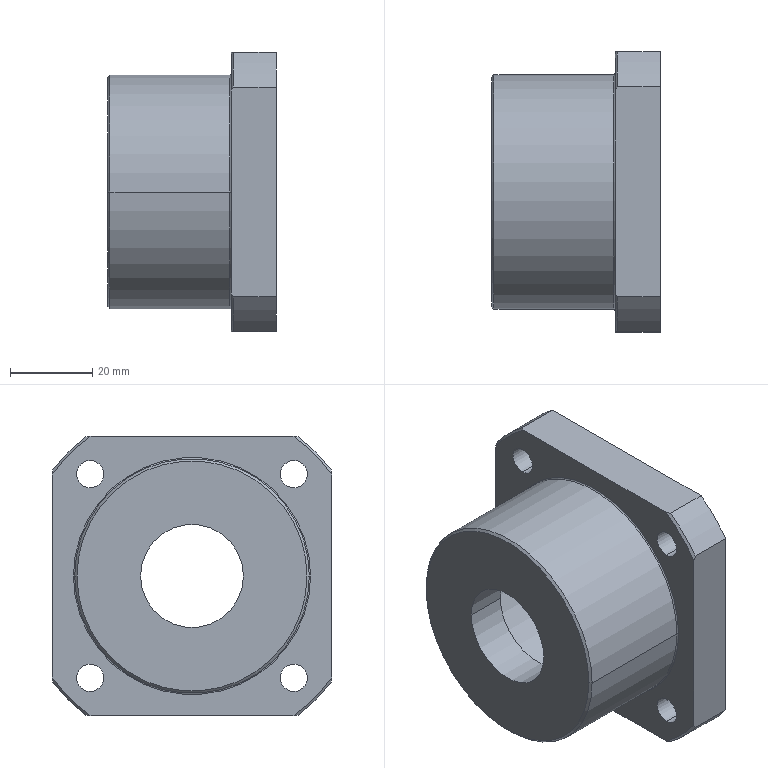Part | NX | 1 solid | 34 faces | box 41 x 68 x 68 mm | volume 65747 mm3 | cylinder 18 | plane 8 | cone 6 | torus 2 | commonest cylinder face diameters 6.6 x8 85 x4 25 x2 47 x2 57 x2
STEP:
#1=CARTESIAN_POINT('',(0.,-12.5,0.));
#2=VERTEX_POINT('',#1);
#3=CARTESIAN_POINT('',(0.,12.5,0.));
#4=VERTEX_POINT('',#3);
#5=CARTESIAN_POINT('',(0.,0.,0.));
#6=DIRECTION('',(-1.,0.,0.));
#7=DIRECTION('',(0.,1.,0.));
#8=AXIS2_PLACEMENT_3D('',#5,#6,#7);
#9=CIRCLE('',#8,12.5);
#10=EDGE_CURVE('',#2,#4,#9,.T.);
#11=ORIENTED_EDGE('',*,*,#10,.T.);
#12=CARTESIAN_POINT('',(10.,12.5,0.));
#13=VERTEX_POINT('',#12);
#14=CARTESIAN_POINT('',(5.,12.5,0.));
#15=DIRECTION('',(1.,0.,0.));
#16=VECTOR('',#15,1000.);
#17=LINE('',#14,#16);
#18=EDGE_CURVE('',#4,#13,#17,.T.);
#19=ORIENTED_EDGE('',*,*,#18,.T.);
#20=CARTESIAN_POINT('',(10.,-12.5,0.));
#21=VERTEX_POINT('',#20);
#22=CARTESIAN_POINT('',(10.,0.,0.));
#23=DIRECTION('',(-1.,0.,0.));
#24=DIRECTION('',(0.,1.,0.));
#25=AXIS2_PLACEMENT_3D('',#22,#23,#24);
#26=CIRCLE('',#25,12.5);
#27=EDGE_CURVE('',#21,#13,#26,.T.);
#28=ORIENTED_EDGE('',*,*,#27,.F.);
#29=CARTESIAN_POINT('',(5.,-12.5,0.));
#30=DIRECTION('',(1.,0.,0.));
#31=VECTOR('',#30,1000.);
#32=LINE('',#29,#31);
#33=EDGE_CURVE('',#2,#21,#32,.T.);
#34=ORIENTED_EDGE('',*,*,#33,.F.);
#35=EDGE_LOOP('',(#11,#19,#28,#34));
#36=FACE_BOUND('',#35,.T.);
#37=CARTESIAN_POINT('',(5.,0.,0.));
#38=DIRECTION('',(1.,0.,0.));
#39=DIRECTION('',(0.,1.,0.));
#40=AXIS2_PLACEMENT_3D('',#37,#38,#39);
#41=CYLINDRICAL_SURFACE('',#40,12.5);
#42=ADVANCED_FACE('',(#36),#41,.F.);
#43=CARTESIAN_POINT('',(0.,-27.93,0.));
#44=VERTEX_POINT('',#43);
#45=CARTESIAN_POINT('',(0.,27.93,0.));
#46=VERTEX_POINT('',#45);
#47=CARTESIAN_POINT('',(0.,0.,0.));
#48=DIRECTION('',(-1.,0.,0.));
#49=DIRECTION('',(0.,1.,0.));
#50=AXIS2_PLACEMENT_3D('',#47,#48,#49);
#51=CIRCLE('',#50,27.93);
#52=EDGE_CURVE('',#44,#46,#51,.T.);
#53=ORIENTED_EDGE('',*,*,#52,.F.);
#54=CARTESIAN_POINT('',(0.57,-28.5,0.));
#55=VERTEX_POINT('',#54);
#56=CARTESIAN_POINT('',(0.285,-28.215,0.));
#57=DIRECTION('',(0.7071,-0.7071,0.));
#58=VECTOR('',#57,1000.);
#59=LINE('',#56,#58);
#60=EDGE_CURVE('',#55,#44,#59,.F.);
#61=ORIENTED_EDGE('',*,*,#60,.F.);
#62=CARTESIAN_POINT('',(0.57,28.5,0.));
#63=VERTEX_POINT('',#62);
#64=CARTESIAN_POINT('',(0.57,0.,0.));
#65=DIRECTION('',(-1.,0.,0.));
#66=DIRECTION('',(0.,1.,0.));
#67=AXIS2_PLACEMENT_3D('',#64,#65,#66);
#68=CIRCLE('',#67,28.5);
#69=EDGE_CURVE('',#55,#63,#68,.T.);
#70=ORIENTED_EDGE('',*,*,#69,.T.);
#71=CARTESIAN_POINT('',(0.285,28.215,0.));
#72=DIRECTION('',(0.7071,0.7071,0.));
#73=VECTOR('',#72,1000.);
#74=LINE('',#71,#73);
#75=EDGE_CURVE('',#63,#46,#74,.F.);
#76=ORIENTED_EDGE('',*,*,#75,.T.);
#77=EDGE_LOOP('',(#53,#61,#70,#76));
#78=FACE_BOUND('',#77,.T.);
#79=CARTESIAN_POINT('',(0.285,0.,0.));
#80=DIRECTION('',(1.,0.,0.));
#81=DIRECTION('',(0.,-1.,0.));
#82=AXIS2_PLACEMENT_3D('',#79,#80,#81);
#83=CONICAL_SURFACE('',#82,28.215,0.7854);
#84=ADVANCED_FACE('',(#78),#83,.T.);
#85=CARTESIAN_POINT('',(0.57,0.,0.));
#86=DIRECTION('',(-1.,0.,0.));
#87=DIRECTION('',(0.,1.,0.));
#88=AXIS2_PLACEMENT_3D('',#85,#86,#87);
#89=CIRCLE('',#88,28.5);
#90=EDGE_CURVE('',#63,#55,#89,.T.);
#91=ORIENTED_EDGE('',*,*,#90,.F.);
#92=CARTESIAN_POINT('',(29.7,28.5,0.));
#93=VERTEX_POINT('',#92);
#94=CARTESIAN_POINT('',(15.135,28.5,0.));
#95=DIRECTION('',(1.,0.,0.));
#96=VECTOR('',#95,1000.);
#97=LINE('',#94,#96);
#98=EDGE_CURVE('',#63,#93,#97,.T.);
#99=ORIENTED_EDGE('',*,*,#98,.T.);
#100=CARTESIAN_POINT('',(29.7,-28.5,0.));
#101=VERTEX_POINT('',#100);
#102=CARTESIAN_POINT('',(29.7,0.,0.));
#103=DIRECTION('',(-1.,0.,0.));
#104=DIRECTION('',(0.,1.,0.));
#105=AXIS2_PLACEMENT_3D('',#102,#103,#104);
#106=CIRCLE('',#105,28.5);
#107=EDGE_CURVE('',#93,#101,#106,.T.);
#108=ORIENTED_EDGE('',*,*,#107,.T.);
#109=CARTESIAN_POINT('',(15.135,-28.5,0.));
#110=DIRECTION('',(1.,0.,0.));
#111=VECTOR('',#110,1000.);
#112=LINE('',#109,#111);
#113=EDGE_CURVE('',#55,#101,#112,.T.);
#114=ORIENTED_EDGE('',*,*,#113,.F.);
#115=EDGE_LOOP('',(#91,#99,#108,#114));
#116=FACE_BOUND('',#115,.T.);
#117=CARTESIAN_POINT('',(15.135,0.,0.));
#118=DIRECTION('',(1.,0.,0.));
#119=DIRECTION('',(0.,1.,0.));
#120=AXIS2_PLACEMENT_3D('',#117,#118,#119);
#121=CYLINDRICAL_SURFACE('',#120,28.5);
#122=ADVANCED_FACE('',(#116),#121,.T.);
#123=ORIENTED_EDGE('',*,*,#107,.F.);
#124=CARTESIAN_POINT('',(30.,28.8,0.));
#125=VERTEX_POINT('',#124);
#126=CARTESIAN_POINT('',(29.7,28.8,0.));
#127=DIRECTION('',(0.,0.,-1.));
#128=DIRECTION('',(-1.,0.,0.));
#129=AXIS2_PLACEMENT_3D('',#126,#127,#128);
#130=CIRCLE('',#129,0.3);
#131=EDGE_CURVE('',#125,#93,#130,.T.);
#132=ORIENTED_EDGE('',*,*,#131,.F.);
#133=CARTESIAN_POINT('',(30.,-28.8,0.));
#134=VERTEX_POINT('',#133);
#135=CARTESIAN_POINT('',(30.,0.,0.));
#136=DIRECTION('',(-1.,0.,0.));
#137=DIRECTION('',(0.,1.,0.));
#138=AXIS2_PLACEMENT_3D('',#135,#136,#137);
#139=CIRCLE('',#138,28.8);
#140=EDGE_CURVE('',#125,#134,#139,.T.);
#141=ORIENTED_EDGE('',*,*,#140,.T.);
#142=CARTESIAN_POINT('',(29.7,-28.8,0.));
#143=DIRECTION('',(0.,0.,1.));
#144=DIRECTION('',(-1.,0.,0.));
#145=AXIS2_PLACEMENT_3D('',#142,#143,#144);
#146=CIRCLE('',#145,0.3);
#147=EDGE_CURVE('',#134,#101,#146,.T.);
#148=ORIENTED_EDGE('',*,*,#147,.T.);
#149=EDGE_LOOP('',(#123,#132,#141,#148));
#150=FACE_BOUND('',#149,.T.);
#151=CARTESIAN_POINT('',(29.7,0.,0.));
#152=DIRECTION('',(-1.,0.,0.));
#153=DIRECTION('',(0.,1.,0.));
#154=AXIS2_PLACEMENT_3D('',#151,#152,#153);
#155=TOROIDAL_SURFACE('',#154,28.8,0.3);
#156=ADVANCED_FACE('',(#150),#155,.F.);
#157=CARTESIAN_POINT('',(10.,23.5,0.));
#158=VERTEX_POINT('',#157);
#159=CARTESIAN_POINT('',(10.,-23.5,0.));
#160=VERTEX_POINT('',#159);
#161=CARTESIAN_POINT('',(10.,0.,0.));
#162=DIRECTION('',(-1.,0.,0.));
#163=DIRECTION('',(0.,1.,0.));
#164=AXIS2_PLACEMENT_3D('',#161,#162,#163);
#165=CIRCLE('',#164,23.5);
#166=EDGE_CURVE('',#158,#160,#165,.T.);
#167=ORIENTED_EDGE('',*,*,#166,.T.);
#168=CARTESIAN_POINT('',(41.,-23.5,0.));
#169=VERTEX_POINT('',#168);
#170=CARTESIAN_POINT('',(25.5,-23.5,0.));
#171=DIRECTION('',(1.,0.,0.));
#172=VECTOR('',#171,1000.);
#173=LINE('',#170,#172);
#174=EDGE_CURVE('',#160,#169,#173,.T.);
#175=ORIENTED_EDGE('',*,*,#174,.T.);
#176=CARTESIAN_POINT('',(41.,23.5,0.));
#177=VERTEX_POINT('',#176);
#178=CARTESIAN_POINT('',(41.,0.,0.));
#179=DIRECTION('',(-1.,0.,0.));
#180=DIRECTION('',(0.,1.,0.));
#181=AXIS2_PLACEMENT_3D('',#178,#179,#180);
#182=CIRCLE('',#181,23.5);
#183=EDGE_CURVE('',#177,#169,#182,.T.);
#184=ORIENTED_EDGE('',*,*,#183,.F.);
#185=CARTESIAN_POINT('',(25.5,23.5,0.));
#186=DIRECTION('',(1.,0.,0.));
#187=VECTOR('',#186,1000.);
#188=LINE('',#185,#187);
#189=EDGE_CURVE('',#158,#177,#188,.T.);
#190=ORIENTED_EDGE('',*,*,#189,.F.);
#191=EDGE_LOOP('',(#167,#175,#184,#190));
#192=FACE_BOUND('',#191,.T.);
#193=CARTESIAN_POINT('',(25.5,0.,0.));
#194=DIRECTION('',(1.,0.,0.));
#195=DIRECTION('',(0.,1.,0.));
#196=AXIS2_PLACEMENT_3D('',#193,#194,#195);
#197=CYLINDRICAL_SURFACE('',#196,23.5);
#198=ADVANCED_FACE('',(#192),#197,.F.);
#199=CARTESIAN_POINT('',(41.,24.749,-28.049));
#200=VERTEX_POINT('',#199);
#201=CARTESIAN_POINT('',(41.,24.749,-21.449));
#202=VERTEX_POINT('',#201);
#203=CARTESIAN_POINT('',(41.,24.749,-24.749));
#204=DIRECTION('',(-1.,0.,0.));
#205=DIRECTION('',(0.,0.,-1.));
#206=AXIS2_PLACEMENT_3D('',#203,#204,#205);
#207=CIRCLE('',#206,3.3);
#208=EDGE_CURVE('',#200,#202,#207,.T.);
#209=ORIENTED_EDGE('',*,*,#208,.F.);
#210=CARTESIAN_POINT('',(30.,24.749,-28.049));
#211=VERTEX_POINT('',#210);
#212=CARTESIAN_POINT('',(52.,24.749,-28.049));
#213=DIRECTION('',(1.,0.,0.));
#214=VECTOR('',#213,1000.);
#215=LINE('',#212,#214);
#216=EDGE_CURVE('',#200,#211,#215,.F.);
#217=ORIENTED_EDGE('',*,*,#216,.T.);
#218=CARTESIAN_POINT('',(30.,24.749,-21.449));
#219=VERTEX_POINT('',#218);
#220=CARTESIAN_POINT('',(30.,24.749,-24.749));
#221=DIRECTION('',(1.,0.,0.));
#222=DIRECTION('',(0.,0.,-1.));
#223=AXIS2_PLACEMENT_3D('',#220,#221,#222);
#224=CIRCLE('',#223,3.3);
#225=EDGE_CURVE('',#219,#211,#224,.T.);
#226=ORIENTED_EDGE('',*,*,#225,.F.);
#227=CARTESIAN_POINT('',(52.,24.749,-21.449));
#228=DIRECTION('',(1.,0.,0.));
#229=VECTOR('',#228,1000.);
#230=LINE('',#227,#229);
#231=EDGE_CURVE('',#202,#219,#230,.F.);
#232=ORIENTED_EDGE('',*,*,#231,.F.);
#233=EDGE_LOOP('',(#209,#217,#226,#232));
#234=FACE_BOUND('',#233,.T.);
#235=CARTESIAN_POINT('',(52.,24.749,-24.749));
#236=DIRECTION('',(1.,0.,0.));
#237=DIRECTION('',(0.,0.,-1.));
#238=AXIS2_PLACEMENT_3D('',#235,#236,#237);
#239=CYLINDRICAL_SURFACE('',#238,3.3);
#240=ADVANCED_FACE('',(#234),#239,.F.);
#241=CARTESIAN_POINT('',(41.,-24.749,-21.449));
#242=VERTEX_POINT('',#241);
#243=CARTESIAN_POINT('',(41.,-24.749,-28.049));
#244=VERTEX_POINT('',#243);
#245=CARTESIAN_POINT('',(41.,-24.749,-24.749));
#246=DIRECTION('',(-1.,0.,0.));
#247=DIRECTION('',(0.,0.,-1.));
#248=AXIS2_PLACEMENT_3D('',#245,#246,#247);
#249=CIRCLE('',#248,3.3);
#250=EDGE_CURVE('',#242,#244,#249,.T.);
#251=ORIENTED_EDGE('',*,*,#250,.F.);
#252=CARTESIAN_POINT('',(30.,-24.749,-21.449));
#253=VERTEX_POINT('',#252);
#254=CARTESIAN_POINT('',(52.,-24.749,-21.449));
#255=DIRECTION('',(1.,0.,0.));
#256=VECTOR('',#255,1000.);
#257=LINE('',#254,#256);
#258=EDGE_CURVE('',#253,#242,#257,.T.);
#259=ORIENTED_EDGE('',*,*,#258,.F.);
#260=CARTESIAN_POINT('',(30.,-24.749,-28.049));
#261=VERTEX_POINT('',#260);
#262=CARTESIAN_POINT('',(30.,-24.749,-24.749));
#263=DIRECTION('',(1.,0.,0.));
#264=DIRECTION('',(0.,0.,-1.));
#265=AXIS2_PLACEMENT_3D('',#262,#263,#264);
#266=CIRCLE('',#265,3.3);
#267=EDGE_CURVE('',#261,#253,#266,.T.);
#268=ORIENTED_EDGE('',*,*,#267,.F.);
#269=CARTESIAN_POINT('',(52.,-24.749,-28.049));
#270=DIRECTION('',(1.,0.,0.));
#271=VECTOR('',#270,1000.);
#272=LINE('',#269,#271);
#273=EDGE_CURVE('',#261,#244,#272,.T.);
#274=ORIENTED_EDGE('',*,*,#273,.T.);
#275=EDGE_LOOP('',(#251,#259,#268,#274));
#276=FACE_BOUND('',#275,.T.);
#277=CARTESIAN_POINT('',(52.,-24.749,-24.749));
#278=DIRECTION('',(1.,0.,0.));
#279=DIRECTION('',(0.,0.,-1.));
#280=AXIS2_PLACEMENT_3D('',#277,#278,#279);
#281=CYLINDRICAL_SURFACE('',#280,3.3);
#282=ADVANCED_FACE('',(#276),#281,.F.);
#283=CARTESIAN_POINT('',(41.,24.749,28.049));
#284=VERTEX_POINT('',#283);
#285=CARTESIAN_POINT('',(41.,24.749,21.449));
#286=VERTEX_POINT('',#285);
#287=CARTESIAN_POINT('',(41.,24.749,24.749));
#288=DIRECTION('',(-1.,0.,0.));
#289=DIRECTION('',(0.,0.,-1.));
#290=AXIS2_PLACEMENT_3D('',#287,#288,#289);
#291=CIRCLE('',#290,3.3);
#292=EDGE_CURVE('',#284,#286,#291,.T.);
#293=ORIENTED_EDGE('',*,*,#292,.F.);
#294=CARTESIAN_POINT('',(30.,24.749,28.049));
#295=VERTEX_POINT('',#294);
#296=CARTESIAN_POINT('',(52.,24.749,28.049));
#297=DIRECTION('',(1.,0.,0.));
#298=VECTOR('',#297,1000.);
#299=LINE('',#296,#298);
#300=EDGE_CURVE('',#284,#295,#299,.F.);
#301=ORIENTED_EDGE('',*,*,#300,.T.);
#302=CARTESIAN_POINT('',(30.,24.749,21.449));
#303=VERTEX_POINT('',#302);
#304=CARTESIAN_POINT('',(30.,24.749,24.749));
#305=DIRECTION('',(1.,0.,0.));
#306=DIRECTION('',(0.,0.,-1.));
#307=AXIS2_PLACEMENT_3D('',#304,#305,#306);
#308=CIRCLE('',#307,3.3);
#309=EDGE_CURVE('',#303,#295,#308,.T.);
#310=ORIENTED_EDGE('',*,*,#309,.F.);
#311=CARTESIAN_POINT('',(52.,24.749,21.449));
#312=DIRECTION('',(1.,0.,0.));
#313=VECTOR('',#312,1000.);
#314=LINE('',#311,#313);
#315=EDGE_CURVE('',#286,#303,#314,.F.);
#316=ORIENTED_EDGE('',*,*,#315,.F.);
#317=EDGE_LOOP('',(#293,#301,#310,#316));
#318=FACE_BOUND('',#317,.T.);
#319=CARTESIAN_POINT('',(52.,24.749,24.749));
#320=DIRECTION('',(1.,0.,0.));
#321=DIRECTION('',(0.,0.,-1.));
#322=AXIS2_PLACEMENT_3D('',#319,#320,#321);
#323=CYLINDRICAL_SURFACE('',#322,3.3);
#324=ADVANCED_FACE('',(#318),#323,.F.);
#325=CARTESIAN_POINT('',(41.,-24.749,28.049));
#326=VERTEX_POINT('',#325);
#327=CARTESIAN_POINT('',(41.,-24.749,21.449));
#328=VERTEX_POINT('',#327);
#329=CARTESIAN_POINT('',(41.,-24.749,24.749));
#330=DIRECTION('',(-1.,0.,0.));
#331=DIRECTION('',(0.,0.,-1.));
#332=AXIS2_PLACEMENT_3D('',#329,#330,#331);
#333=CIRCLE('',#332,3.3);
#334=EDGE_CURVE('',#326,#328,#333,.T.);
#335=ORIENTED_EDGE('',*,*,#334,.F.);
#336=CARTESIAN_POINT('',(30.,-24.749,28.049));
#337=VERTEX_POINT('',#336);
#338=CARTESIAN_POINT('',(52.,-24.749,28.049));
#339=DIRECTION('',(1.,0.,0.));
#340=VECTOR('',#339,1000.);
#341=LINE('',#338,#340);
#342=EDGE_CURVE('',#337,#326,#341,.T.);
#343=ORIENTED_EDGE('',*,*,#342,.F.);
#344=CARTESIAN_POINT('',(30.,-24.749,21.449));
#345=VERTEX_POINT('',#344);
#346=CARTESIAN_POINT('',(30.,-24.749,24.749));
#347=DIRECTION('',(1.,0.,0.));
#348=DIRECTION('',(0.,0.,-1.));
#349=AXIS2_PLACEMENT_3D('',#346,#347,#348);
#350=CIRCLE('',#349,3.3);
#351=EDGE_CURVE('',#345,#337,#350,.T.);
#352=ORIENTED_EDGE('',*,*,#351,.F.);
#353=CARTESIAN_POINT('',(52.,-24.749,21.449));
#354=DIRECTION('',(1.,0.,0.));
#355=VECTOR('',#354,1000.);
#356=LINE('',#353,#355);
#357=EDGE_CURVE('',#345,#328,#356,.T.);
#358=ORIENTED_EDGE('',*,*,#357,.T.);
#359=EDGE_LOOP('',(#335,#343,#352,#358));
#360=FACE_BOUND('',#359,.T.);
#361=CARTESIAN_POINT('',(52.,-24.749,24.749));
#362=DIRECTION('',(1.,0.,0.));
#363=DIRECTION('',(0.,0.,-1.));
#364=AXIS2_PLACEMENT_3D('',#361,#362,#363);
#365=CYLINDRICAL_SURFACE('',#364,3.3);
#366=ADVANCED_FACE('',(#360),#365,.F.);
#367=CARTESIAN_POINT('',(30.57,34.,25.5));
#368=VERTEX_POINT('',#367);
#369=CARTESIAN_POINT('',(30.,34.,24.538));
#370=VERTEX_POINT('',#369);
#371=CARTESIAN_POINT('',(30.57,34.,25.5));
#372=CARTESIAN_POINT('',(30.28,34.,25.016));
#373=CARTESIAN_POINT('',(30.,34.,24.538));
#374=(BOUNDED_CURVE()B_SPLINE_CURVE(2,(#371,#372,#373),.UNSPECIFIED.,.F.,.F.)B_SPLINE_CURVE_WITH_KNOTS((3,3),(0.,1.118),.UNSPECIFIED.)CURVE()GEOMETRIC_REPRESENTATION_ITEM()RATIONAL_B_SPLINE_CURVE((1.,1.,1.))REPRESENTATION_ITEM(''));
#375=EDGE_CURVE('',#368,#370,#374,.T.);
#376=ORIENTED_EDGE('',*,*,#375,.T.);
#377=CARTESIAN_POINT('',(30.,24.538,34.));
#378=VERTEX_POINT('',#377);
#379=CARTESIAN_POINT('',(30.,0.,0.));
#380=DIRECTION('',(-1.,0.,0.));
#381=DIRECTION('',(0.,1.,0.));
#382=AXIS2_PLACEMENT_3D('',#379,#380,#381);
#383=CIRCLE('',#382,41.93);
#384=EDGE_CURVE('',#378,#370,#383,.T.);
#385=ORIENTED_EDGE('',*,*,#384,.F.);
#386=CARTESIAN_POINT('',(30.57,25.5,34.));
#387=VERTEX_POINT('',#386);
#388=CARTESIAN_POINT('',(30.,24.538,34.));
#389=CARTESIAN_POINT('',(30.28,25.016,34.));
#390=CARTESIAN_POINT('',(30.57,25.5,34.));
#391=(BOUNDED_CURVE()B_SPLINE_CURVE(2,(#388,#389,#390),.UNSPECIFIED.,.F.,.F.)B_SPLINE_CURVE_WITH_KNOTS((3,3),(0.,1.118),.UNSPECIFIED.)CURVE()GEOMETRIC_REPRESENTATION_ITEM()RATIONAL_B_SPLINE_CURVE((1.,1.,1.))REPRESENTATION_ITEM(''));
#392=EDGE_CURVE('',#378,#387,#391,.T.);
#393=ORIENTED_EDGE('',*,*,#392,.T.);
#394=CARTESIAN_POINT('',(30.57,0.,0.));
#395=DIRECTION('',(-1.,0.,0.));
#396=DIRECTION('',(0.,1.,0.));
#397=AXIS2_PLACEMENT_3D('',#394,#395,#396);
#398=CIRCLE('',#397,42.5);
#399=EDGE_CURVE('',#387,#368,#398,.T.);
#400=ORIENTED_EDGE('',*,*,#399,.T.);
#401=EDGE_LOOP('',(#376,#385,#393,#400));
#402=FACE_BOUND('',#401,.T.);
#403=CARTESIAN_POINT('',(30.285,0.,0.));
#404=DIRECTION('',(1.,0.,0.));
#405=DIRECTION('',(0.,-1.,0.));
#406=AXIS2_PLACEMENT_3D('',#403,#404,#405);
#407=CONICAL_SURFACE('',#406,42.215,0.7854);
#408=ADVANCED_FACE('',(#402),#407,.T.);
#409=CARTESIAN_POINT('',(41.,34.,25.5));
#410=VERTEX_POINT('',#409);
#411=CARTESIAN_POINT('',(35.785,34.,25.5));
#412=DIRECTION('',(-1.,0.,0.));
#413=VECTOR('',#412,1000.);
#414=LINE('',#411,#413);
#415=EDGE_CURVE('',#410,#368,#414,.T.);
#416=ORIENTED_EDGE('',*,*,#415,.T.);
#417=ORIENTED_EDGE('',*,*,#399,.F.);
#418=CARTESIAN_POINT('',(41.,25.5,34.));
#419=VERTEX_POINT('',#418);
#420=CARTESIAN_POINT('',(35.785,25.5,34.));
#421=DIRECTION('',(1.,0.,0.));
#422=VECTOR('',#421,1000.);
#423=LINE('',#420,#422);
#424=EDGE_CURVE('',#387,#419,#423,.T.);
#425=ORIENTED_EDGE('',*,*,#424,.T.);
#426=CARTESIAN_POINT('',(41.,0.,0.));
#427=DIRECTION('',(-1.,0.,0.));
#428=DIRECTION('',(0.,1.,0.));
#429=AXIS2_PLACEMENT_3D('',#426,#427,#428);
#430=CIRCLE('',#429,42.5);
#431=EDGE_CURVE('',#419,#410,#430,.T.);
#432=ORIENTED_EDGE('',*,*,#431,.T.);
#433=EDGE_LOOP('',(#416,#417,#425,#432));
#434=FACE_BOUND('',#433,.T.);
#435=CARTESIAN_POINT('',(35.785,0.,0.));
#436=DIRECTION('',(1.,0.,0.));
#437=DIRECTION('',(0.,1.,0.));
#438=AXIS2_PLACEMENT_3D('',#435,#436,#437);
#439=CYLINDRICAL_SURFACE('',#438,42.5);
#440=ADVANCED_FACE('',(#434),#439,.T.);
#441=ORIENTED_EDGE('',*,*,#52,.T.);
#442=CARTESIAN_POINT('',(0.,0.,0.));
#443=DIRECTION('',(-1.,0.,0.));
#444=DIRECTION('',(0.,1.,0.));
#445=AXIS2_PLACEMENT_3D('',#442,#443,#444);
#446=CIRCLE('',#445,27.93);
#447=EDGE_CURVE('',#46,#44,#446,.T.);
#448=ORIENTED_EDGE('',*,*,#447,.T.);
#449=EDGE_LOOP('',(#441,#448));
#450=FACE_BOUND('',#449,.T.);
#451=ORIENTED_EDGE('',*,*,#10,.F.);
#452=CARTESIAN_POINT('',(0.,0.,0.));
#453=DIRECTION('',(-1.,0.,0.));
#454=DIRECTION('',(0.,1.,0.));
#455=AXIS2_PLACEMENT_3D('',#452,#453,#454);
#456=CIRCLE('',#455,12.5);
#457=EDGE_CURVE('',#4,#2,#456,.T.);
#458=ORIENTED_EDGE('',*,*,#457,.F.);
#459=EDGE_LOOP('',(#451,#458));
#460=FACE_BOUND('',#459,.T.);
#461=CARTESIAN_POINT('',(0.,20.215,0.));
#462=DIRECTION('',(-1.,0.,0.));
#463=DIRECTION('',(0.,0.,1.));
#464=AXIS2_PLACEMENT_3D('',#461,#462,#463);
#465=PLANE('',#464);
#466=ADVANCED_FACE('',(#450,#460),#465,.T.);
#467=CARTESIAN_POINT('',(41.,34.,-25.5));
#468=VERTEX_POINT('',#467);
#469=CARTESIAN_POINT('',(41.,34.,17.));
#470=DIRECTION('',(0.,0.,1.));
#471=VECTOR('',#470,1000.);
#472=LINE('',#469,#471);
#473=EDGE_CURVE('',#468,#410,#472,.T.);
#474=ORIENTED_EDGE('',*,*,#473,.T.);
#475=ORIENTED_EDGE('',*,*,#431,.F.);
#476=CARTESIAN_POINT('',(41.,-25.5,34.));
#477=VERTEX_POINT('',#476);
#478=CARTESIAN_POINT('',(41.,-0.5,34.));
#479=DIRECTION('',(0.,-1.,0.));
#480=VECTOR('',#479,1000.);
#481=LINE('',#478,#480);
#482=EDGE_CURVE('',#419,#477,#481,.T.);
#483=ORIENTED_EDGE('',*,*,#482,.T.);
#484=CARTESIAN_POINT('',(41.,-34.,25.5));
#485=VERTEX_POINT('',#484);
#486=CARTESIAN_POINT('',(41.,0.,0.));
#487=DIRECTION('',(-1.,0.,0.));
#488=DIRECTION('',(0.,1.,0.));
#489=AXIS2_PLACEMENT_3D('',#486,#487,#488);
#490=CIRCLE('',#489,42.5);
#491=EDGE_CURVE('',#485,#477,#490,.T.);
#492=ORIENTED_EDGE('',*,*,#491,.F.);
#493=CARTESIAN_POINT('',(41.,-34.,-25.5));
#494=VERTEX_POINT('',#493);
#495=CARTESIAN_POINT('',(41.,-34.,-17.));
#496=DIRECTION('',(0.,0.,-1.));
#497=VECTOR('',#496,1000.);
#498=LINE('',#495,#497);
#499=EDGE_CURVE('',#485,#494,#498,.T.);
#500=ORIENTED_EDGE('',*,*,#499,.T.);
#501=CARTESIAN_POINT('',(41.,-25.5,-34.));
#502=VERTEX_POINT('',#501);
#503=CARTESIAN_POINT('',(41.,0.,0.));
#504=DIRECTION('',(-1.,0.,0.));
#505=DIRECTION('',(0.,1.,0.));
#506=AXIS2_PLACEMENT_3D('',#503,#504,#505);
#507=CIRCLE('',#506,42.5);
#508=EDGE_CURVE('',#502,#494,#507,.T.);
#509=ORIENTED_EDGE('',*,*,#508,.F.);
#510=CARTESIAN_POINT('',(41.,25.5,-34.));
#511=VERTEX_POINT('',#510);
#512=CARTESIAN_POINT('',(41.,33.5,-34.));
#513=DIRECTION('',(0.,1.,0.));
#514=VECTOR('',#513,1000.);
#515=LINE('',#512,#514);
#516=EDGE_CURVE('',#502,#511,#515,.T.);
#517=ORIENTED_EDGE('',*,*,#516,.T.);
#518=CARTESIAN_POINT('',(41.,0.,0.));
#519=DIRECTION('',(-1.,0.,0.));
#520=DIRECTION('',(0.,1.,0.));
#521=AXIS2_PLACEMENT_3D('',#518,#519,#520);
#522=CIRCLE('',#521,42.5);
#523=EDGE_CURVE('',#468,#511,#522,.T.);
#524=ORIENTED_EDGE('',*,*,#523,.F.);
#525=EDGE_LOOP('',(#474,#475,#483,#492,#500,#509,#517,#524));
#526=FACE_BOUND('',#525,.T.);
#527=ORIENTED_EDGE('',*,*,#334,.T.);
#528=CARTESIAN_POINT('',(41.,-24.749,24.749));
#529=DIRECTION('',(-1.,0.,0.));
#530=DIRECTION('',(0.,0.,-1.));
#531=AXIS2_PLACEMENT_3D('',#528,#529,#530);
#532=CIRCLE('',#531,3.3);
#533=EDGE_CURVE('',#328,#326,#532,.T.);
#534=ORIENTED_EDGE('',*,*,#533,.T.);
#535=EDGE_LOOP('',(#527,#534));
#536=FACE_BOUND('',#535,.T.);
#537=ORIENTED_EDGE('',*,*,#292,.T.);
#538=CARTESIAN_POINT('',(41.,24.749,24.749));
#539=DIRECTION('',(-1.,0.,0.));
#540=DIRECTION('',(0.,0.,-1.));
#541=AXIS2_PLACEMENT_3D('',#538,#539,#540);
#542=CIRCLE('',#541,3.3);
#543=EDGE_CURVE('',#286,#284,#542,.T.);
#544=ORIENTED_EDGE('',*,*,#543,.T.);
#545=EDGE_LOOP('',(#537,#544));
#546=FACE_BOUND('',#545,.T.);
#547=ORIENTED_EDGE('',*,*,#250,.T.);
#548=CARTESIAN_POINT('',(41.,-24.749,-24.749));
#549=DIRECTION('',(-1.,0.,0.));
#550=DIRECTION('',(0.,0.,-1.));
#551=AXIS2_PLACEMENT_3D('',#548,#549,#550);
#552=CIRCLE('',#551,3.3);
#553=EDGE_CURVE('',#244,#242,#552,.T.);
#554=ORIENTED_EDGE('',*,*,#553,.T.);
#555=EDGE_LOOP('',(#547,#554));
#556=FACE_BOUND('',#555,.T.);
#557=ORIENTED_EDGE('',*,*,#208,.T.);
#558=CARTESIAN_POINT('',(41.,24.749,-24.749));
#559=DIRECTION('',(-1.,0.,0.));
#560=DIRECTION('',(0.,0.,-1.));
#561=AXIS2_PLACEMENT_3D('',#558,#559,#560);
#562=CIRCLE('',#561,3.3);
#563=EDGE_CURVE('',#202,#200,#562,.T.);
#564=ORIENTED_EDGE('',*,*,#563,.T.);
#565=EDGE_LOOP('',(#557,#564));
#566=FACE_BOUND('',#565,.T.);
#567=ORIENTED_EDGE('',*,*,#183,.T.);
#568=CARTESIAN_POINT('',(41.,0.,0.));
#569=DIRECTION('',(-1.,0.,0.));
#570=DIRECTION('',(0.,1.,0.));
#571=AXIS2_PLACEMENT_3D('',#568,#569,#570);
#572=CIRCLE('',#571,23.5);
#573=EDGE_CURVE('',#169,#177,#572,.T.);
#574=ORIENTED_EDGE('',*,*,#573,.T.);
#575=EDGE_LOOP('',(#567,#574));
#576=FACE_BOUND('',#575,.T.);
#577=CARTESIAN_POINT('',(41.,33.,0.));
#578=DIRECTION('',(1.,0.,0.));
#579=DIRECTION('',(0.,1.,0.));
#580=AXIS2_PLACEMENT_3D('',#577,#578,#579);
#581=PLANE('',#580);
#582=ADVANCED_FACE('',(#526,#536,#546,#556,#566,#576),#581,.T.);
#583=ORIENTED_EDGE('',*,*,#375,.F.);
#584=ORIENTED_EDGE('',*,*,#415,.F.);
#585=ORIENTED_EDGE('',*,*,#473,.F.);
#586=CARTESIAN_POINT('',(30.57,34.,-25.5));
#587=VERTEX_POINT('',#586);
#588=CARTESIAN_POINT('',(35.785,34.,-25.5));
#589=DIRECTION('',(1.,0.,0.));
#590=VECTOR('',#589,1000.);
#591=LINE('',#588,#590);
#592=EDGE_CURVE('',#587,#468,#591,.T.);
#593=ORIENTED_EDGE('',*,*,#592,.F.);
#594=CARTESIAN_POINT('',(30.,34.,-24.538));
#595=VERTEX_POINT('',#594);
#596=CARTESIAN_POINT('',(30.,34.,-24.538));
#597=CARTESIAN_POINT('',(30.28,34.,-25.016));
#598=CARTESIAN_POINT('',(30.57,34.,-25.5));
#599=(BOUNDED_CURVE()B_SPLINE_CURVE(2,(#596,#597,#598),.UNSPECIFIED.,.F.,.F.)B_SPLINE_CURVE_WITH_KNOTS((3,3),(0.,1.118),.UNSPECIFIED.)CURVE()GEOMETRIC_REPRESENTATION_ITEM()RATIONAL_B_SPLINE_CURVE((1.,1.,1.))REPRESENTATION_ITEM(''));
#600=EDGE_CURVE('',#595,#587,#599,.T.);
#601=ORIENTED_EDGE('',*,*,#600,.F.);
#602=CARTESIAN_POINT('',(30.,34.,17.));
#603=DIRECTION('',(0.,0.,-1.));
#604=VECTOR('',#603,1000.);
#605=LINE('',#602,#604);
#606=EDGE_CURVE('',#370,#595,#605,.T.);
#607=ORIENTED_EDGE('',*,*,#606,.F.);
#608=EDGE_LOOP('',(#583,#584,#585,#593,#601,#607));
#609=FACE_BOUND('',#608,.T.);
#610=CARTESIAN_POINT('',(52.,34.,34.));
#611=DIRECTION('',(0.,-1.,0.));
#612=DIRECTION('',(0.,0.,-1.));
#613=AXIS2_PLACEMENT_3D('',#610,#611,#612);
#614=PLANE('',#613);
#615=ADVANCED_FACE('',(#609),#614,.F.);
#616=CARTESIAN_POINT('',(30.57,25.5,-34.));
#617=VERTEX_POINT('',#616);
#618=CARTESIAN_POINT('',(30.,24.538,-34.));
#619=VERTEX_POINT('',#618);
#620=CARTESIAN_POINT('',(30.57,25.5,-34.));
#621=CARTESIAN_POINT('',(30.28,25.016,-34.));
#622=CARTESIAN_POINT('',(30.,24.538,-34.));
#623=(BOUNDED_CURVE()B_SPLINE_CURVE(2,(#620,#621,#622),.UNSPECIFIED.,.F.,.F.)B_SPLINE_CURVE_WITH_KNOTS((3,3),(0.,1.118),.UNSPECIFIED.)CURVE()GEOMETRIC_REPRESENTATION_ITEM()RATIONAL_B_SPLINE_CURVE((1.,1.,1.))REPRESENTATION_ITEM(''));
#624=EDGE_CURVE('',#617,#619,#623,.T.);
#625=ORIENTED_EDGE('',*,*,#624,.F.);
#626=CARTESIAN_POINT('',(35.785,25.5,-34.));
#627=DIRECTION('',(-1.,0.,0.));
#628=VECTOR('',#627,1000.);
#629=LINE('',#626,#628);
#630=EDGE_CURVE('',#511,#617,#629,.T.);
#631=ORIENTED_EDGE('',*,*,#630,.F.);
#632=ORIENTED_EDGE('',*,*,#516,.F.);
#633=CARTESIAN_POINT('',(30.57,-25.5,-34.));
#634=VERTEX_POINT('',#633);
#635=CARTESIAN_POINT('',(35.785,-25.5,-34.));
#636=DIRECTION('',(1.,0.,0.));
#637=VECTOR('',#636,1000.);
#638=LINE('',#635,#637);
#639=EDGE_CURVE('',#634,#502,#638,.T.);
#640=ORIENTED_EDGE('',*,*,#639,.F.);
#641=CARTESIAN_POINT('',(30.,-24.538,-34.));
#642=VERTEX_POINT('',#641);
#643=CARTESIAN_POINT('',(30.,-24.538,-34.));
#644=CARTESIAN_POINT('',(30.28,-25.016,-34.));
#645=CARTESIAN_POINT('',(30.57,-25.5,-34.));
#646=(BOUNDED_CURVE()B_SPLINE_CURVE(2,(#643,#644,#645),.UNSPECIFIED.,.F.,.F.)B_SPLINE_CURVE_WITH_KNOTS((3,3),(0.,1.118),.UNSPECIFIED.)CURVE()GEOMETRIC_REPRESENTATION_ITEM()RATIONAL_B_SPLINE_CURVE((1.,1.,1.))REPRESENTATION_ITEM(''));
#647=EDGE_CURVE('',#642,#634,#646,.T.);
#648=ORIENTED_EDGE('',*,*,#647,.F.);
#649=CARTESIAN_POINT('',(30.,34.682,-34.));
#650=DIRECTION('',(0.,-1.,0.));
#651=VECTOR('',#650,1000.);
#652=LINE('',#649,#651);
#653=EDGE_CURVE('',#619,#642,#652,.T.);
#654=ORIENTED_EDGE('',*,*,#653,.F.);
#655=EDGE_LOOP('',(#625,#631,#632,#640,#648,#654));
#656=FACE_BOUND('',#655,.T.);
#657=CARTESIAN_POINT('',(52.,34.,-34.));
#658=DIRECTION('',(0.,0.,1.));
#659=DIRECTION('',(1.,0.,0.));
#660=AXIS2_PLACEMENT_3D('',#657,#658,#659);
#661=PLANE('',#660);
#662=ADVANCED_FACE('',(#656),#661,.F.);
#663=CARTESIAN_POINT('',(30.57,-34.,-25.5));
#664=VERTEX_POINT('',#663);
#665=CARTESIAN_POINT('',(30.,-34.,-24.538));
#666=VERTEX_POINT('',#665);
#667=CARTESIAN_POINT('',(30.57,-34.,-25.5));
#668=CARTESIAN_POINT('',(30.28,-34.,-25.016));
#669=CARTESIAN_POINT('',(30.,-34.,-24.538));
#670=(BOUNDED_CURVE()B_SPLINE_CURVE(2,(#667,#668,#669),.UNSPECIFIED.,.F.,.F.)B_SPLINE_CURVE_WITH_KNOTS((3,3),(0.,1.118),.UNSPECIFIED.)CURVE()GEOMETRIC_REPRESENTATION_ITEM()RATIONAL_B_SPLINE_CURVE((1.,1.,1.))REPRESENTATION_ITEM(''));
#671=EDGE_CURVE('',#664,#666,#670,.T.);
#672=ORIENTED_EDGE('',*,*,#671,.F.);
#673=CARTESIAN_POINT('',(35.785,-34.,-25.5));
#674=DIRECTION('',(-1.,0.,0.));
#675=VECTOR('',#674,1000.);
#676=LINE('',#673,#675);
#677=EDGE_CURVE('',#494,#664,#676,.T.);
#678=ORIENTED_EDGE('',*,*,#677,.F.);
#679=ORIENTED_EDGE('',*,*,#499,.F.);
#680=CARTESIAN_POINT('',(30.57,-34.,25.5));
#681=VERTEX_POINT('',#680);
#682=CARTESIAN_POINT('',(35.785,-34.,25.5));
#683=DIRECTION('',(1.,0.,0.));
#684=VECTOR('',#683,1000.);
#685=LINE('',#682,#684);
#686=EDGE_CURVE('',#681,#485,#685,.T.);
#687=ORIENTED_EDGE('',*,*,#686,.F.);
#688=CARTESIAN_POINT('',(30.,-34.,24.538));
#689=VERTEX_POINT('',#688);
#690=CARTESIAN_POINT('',(30.,-34.,24.538));
#691=CARTESIAN_POINT('',(30.28,-34.,25.016));
#692=CARTESIAN_POINT('',(30.57,-34.,25.5));
#693=(BOUNDED_CURVE()B_SPLINE_CURVE(2,(#690,#691,#692),.UNSPECIFIED.,.F.,.F.)B_SPLINE_CURVE_WITH_KNOTS((3,3),(0.,1.118),.UNSPECIFIED.)CURVE()GEOMETRIC_REPRESENTATION_ITEM()RATIONAL_B_SPLINE_CURVE((1.,1.,1.))REPRESENTATION_ITEM(''));
#694=EDGE_CURVE('',#689,#681,#693,.T.);
#695=ORIENTED_EDGE('',*,*,#694,.F.);
#696=CARTESIAN_POINT('',(30.,-34.,-17.));
#697=DIRECTION('',(0.,0.,1.));
#698=VECTOR('',#697,1000.);
#699=LINE('',#696,#698);
#700=EDGE_CURVE('',#666,#689,#699,.T.);
#701=ORIENTED_EDGE('',*,*,#700,.F.);
#702=EDGE_LOOP('',(#672,#678,#679,#687,#695,#701));
#703=FACE_BOUND('',#702,.T.);
#704=CARTESIAN_POINT('',(52.,-34.,-34.));
#705=DIRECTION('',(0.,1.,0.));
#706=DIRECTION('',(1.,0.,0.));
#707=AXIS2_PLACEMENT_3D('',#704,#705,#706);
#708=PLANE('',#707);
#709=ADVANCED_FACE('',(#703),#708,.F.);
#710=CARTESIAN_POINT('',(30.57,-25.5,34.));
#711=VERTEX_POINT('',#710);
#712=CARTESIAN_POINT('',(30.,-24.538,34.));
#713=VERTEX_POINT('',#712);
#714=CARTESIAN_POINT('',(30.57,-25.5,34.));
#715=CARTESIAN_POINT('',(30.28,-25.016,34.));
#716=CARTESIAN_POINT('',(30.,-24.538,34.));
#717=(BOUNDED_CURVE()B_SPLINE_CURVE(2,(#714,#715,#716),.UNSPECIFIED.,.F.,.F.)B_SPLINE_CURVE_WITH_KNOTS((3,3),(0.,1.118),.UNSPECIFIED.)CURVE()GEOMETRIC_REPRESENTATION_ITEM()RATIONAL_B_SPLINE_CURVE((1.,1.,1.))REPRESENTATION_ITEM(''));
#718=EDGE_CURVE('',#711,#713,#717,.T.);
#719=ORIENTED_EDGE('',*,*,#718,.F.);
#720=CARTESIAN_POINT('',(35.785,-25.5,34.));
#721=DIRECTION('',(-1.,0.,0.));
#722=VECTOR('',#721,1000.);
#723=LINE('',#720,#722);
#724=EDGE_CURVE('',#477,#711,#723,.T.);
#725=ORIENTED_EDGE('',*,*,#724,.F.);
#726=ORIENTED_EDGE('',*,*,#482,.F.);
#727=ORIENTED_EDGE('',*,*,#424,.F.);
#728=ORIENTED_EDGE('',*,*,#392,.F.);
#729=CARTESIAN_POINT('',(30.,0.6825,34.));
#730=DIRECTION('',(0.,1.,0.));
#731=VECTOR('',#730,1000.);
#732=LINE('',#729,#731);
#733=EDGE_CURVE('',#713,#378,#732,.T.);
#734=ORIENTED_EDGE('',*,*,#733,.F.);
#735=EDGE_LOOP('',(#719,#725,#726,#727,#728,#734));
#736=FACE_BOUND('',#735,.T.);
#737=CARTESIAN_POINT('',(52.,-34.,34.));
#738=DIRECTION('',(0.,0.,-1.));
#739=DIRECTION('',(0.,-1.,0.));
#740=AXIS2_PLACEMENT_3D('',#737,#738,#739);
#741=PLANE('',#740);
#742=ADVANCED_FACE('',(#736),#741,.F.);
#743=ORIENTED_EDGE('',*,*,#606,.T.);
#744=CARTESIAN_POINT('',(30.,0.,0.));
#745=DIRECTION('',(-1.,0.,0.));
#746=DIRECTION('',(0.,1.,0.));
#747=AXIS2_PLACEMENT_3D('',#744,#745,#746);
#748=CIRCLE('',#747,41.93);
#749=EDGE_CURVE('',#595,#619,#748,.T.);
#750=ORIENTED_EDGE('',*,*,#749,.T.);
#751=ORIENTED_EDGE('',*,*,#653,.T.);
#752=CARTESIAN_POINT('',(30.,0.,0.));
#753=DIRECTION('',(-1.,0.,0.));
#754=DIRECTION('',(0.,1.,0.));
#755=AXIS2_PLACEMENT_3D('',#752,#753,#754);
#756=CIRCLE('',#755,41.93);
#757=EDGE_CURVE('',#642,#666,#756,.T.);
#758=ORIENTED_EDGE('',*,*,#757,.T.);
#759=ORIENTED_EDGE('',*,*,#700,.T.);
#760=CARTESIAN_POINT('',(30.,0.,0.));
#761=DIRECTION('',(-1.,0.,0.));
#762=DIRECTION('',(0.,1.,0.));
#763=AXIS2_PLACEMENT_3D('',#760,#761,#762);
#764=CIRCLE('',#763,41.93);
#765=EDGE_CURVE('',#689,#713,#764,.T.);
#766=ORIENTED_EDGE('',*,*,#765,.T.);
#767=ORIENTED_EDGE('',*,*,#733,.T.);
#768=ORIENTED_EDGE('',*,*,#384,.T.);
#769=EDGE_LOOP('',(#743,#750,#751,#758,#759,#766,#767,#768));
#770=FACE_BOUND('',#769,.T.);
#771=CARTESIAN_POINT('',(30.,-24.749,24.749));
#772=DIRECTION('',(1.,0.,0.));
#773=DIRECTION('',(0.,0.,-1.));
#774=AXIS2_PLACEMENT_3D('',#771,#772,#773);
#775=CIRCLE('',#774,3.3);
#776=EDGE_CURVE('',#337,#345,#775,.T.);
#777=ORIENTED_EDGE('',*,*,#776,.T.);
#778=ORIENTED_EDGE('',*,*,#351,.T.);
#779=EDGE_LOOP('',(#777,#778));
#780=FACE_BOUND('',#779,.T.);
#781=ORIENTED_EDGE('',*,*,#309,.T.);
#782=CARTESIAN_POINT('',(30.,24.749,24.749));
#783=DIRECTION('',(1.,0.,0.));
#784=DIRECTION('',(0.,0.,-1.));
#785=AXIS2_PLACEMENT_3D('',#782,#783,#784);
#786=CIRCLE('',#785,3.3);
#787=EDGE_CURVE('',#295,#303,#786,.T.);
#788=ORIENTED_EDGE('',*,*,#787,.T.);
#789=EDGE_LOOP('',(#781,#788));
#790=FACE_BOUND('',#789,.T.);
#791=CARTESIAN_POINT('',(30.,-24.749,-24.749));
#792=DIRECTION('',(1.,0.,0.));
#793=DIRECTION('',(0.,0.,-1.));
#794=AXIS2_PLACEMENT_3D('',#791,#792,#793);
#795=CIRCLE('',#794,3.3);
#796=EDGE_CURVE('',#253,#261,#795,.T.);
#797=ORIENTED_EDGE('',*,*,#796,.T.);
#798=ORIENTED_EDGE('',*,*,#267,.T.);
#799=EDGE_LOOP('',(#797,#798));
#800=FACE_BOUND('',#799,.T.);
#801=ORIENTED_EDGE('',*,*,#225,.T.);
#802=CARTESIAN_POINT('',(30.,24.749,-24.749));
#803=DIRECTION('',(1.,0.,0.));
#804=DIRECTION('',(0.,0.,-1.));
#805=AXIS2_PLACEMENT_3D('',#802,#803,#804);
#806=CIRCLE('',#805,3.3);
#807=EDGE_CURVE('',#211,#219,#806,.T.);
#808=ORIENTED_EDGE('',*,*,#807,.T.);
#809=EDGE_LOOP('',(#801,#808));
#810=FACE_BOUND('',#809,.T.);
#811=ORIENTED_EDGE('',*,*,#140,.F.);
#812=CARTESIAN_POINT('',(30.,0.,0.));
#813=DIRECTION('',(-1.,0.,0.));
#814=DIRECTION('',(0.,1.,0.));
#815=AXIS2_PLACEMENT_3D('',#812,#813,#814);
#816=CIRCLE('',#815,28.8);
#817=EDGE_CURVE('',#134,#125,#816,.T.);
#818=ORIENTED_EDGE('',*,*,#817,.F.);
#819=EDGE_LOOP('',(#811,#818));
#820=FACE_BOUND('',#819,.T.);
#821=CARTESIAN_POINT('',(30.,35.365,0.));
#822=DIRECTION('',(-1.,0.,0.));
#823=DIRECTION('',(0.,0.,1.));
#824=AXIS2_PLACEMENT_3D('',#821,#822,#823);
#825=PLANE('',#824);
#826=ADVANCED_FACE('',(#770,#780,#790,#800,#810,#820),#825,.T.);
#827=ORIENTED_EDGE('',*,*,#647,.T.);
#828=CARTESIAN_POINT('',(30.57,0.,0.));
#829=DIRECTION('',(-1.,0.,0.));
#830=DIRECTION('',(0.,1.,0.));
#831=AXIS2_PLACEMENT_3D('',#828,#829,#830);
#832=CIRCLE('',#831,42.5);
#833=EDGE_CURVE('',#634,#664,#832,.T.);
#834=ORIENTED_EDGE('',*,*,#833,.T.);
#835=ORIENTED_EDGE('',*,*,#671,.T.);
#836=ORIENTED_EDGE('',*,*,#757,.F.);
#837=EDGE_LOOP('',(#827,#834,#835,#836));
#838=FACE_BOUND('',#837,.T.);
#839=CARTESIAN_POINT('',(30.285,0.,0.));
#840=DIRECTION('',(1.,0.,0.));
#841=DIRECTION('',(0.,-1.,0.));
#842=AXIS2_PLACEMENT_3D('',#839,#840,#841);
#843=CONICAL_SURFACE('',#842,42.215,0.7854);
#844=ADVANCED_FACE('',(#838),#843,.T.);
#845=ORIENTED_EDGE('',*,*,#694,.T.);
#846=CARTESIAN_POINT('',(30.57,0.,0.));
#847=DIRECTION('',(-1.,0.,0.));
#848=DIRECTION('',(0.,1.,0.));
#849=AXIS2_PLACEMENT_3D('',#846,#847,#848);
#850=CIRCLE('',#849,42.5);
#851=EDGE_CURVE('',#681,#711,#850,.T.);
#852=ORIENTED_EDGE('',*,*,#851,.T.);
#853=ORIENTED_EDGE('',*,*,#718,.T.);
#854=ORIENTED_EDGE('',*,*,#765,.F.);
#855=EDGE_LOOP('',(#845,#852,#853,#854));
#856=FACE_BOUND('',#855,.T.);
#857=CARTESIAN_POINT('',(30.285,0.,0.));
#858=DIRECTION('',(1.,0.,0.));
#859=DIRECTION('',(0.,-1.,0.));
#860=AXIS2_PLACEMENT_3D('',#857,#858,#859);
#861=CONICAL_SURFACE('',#860,42.215,0.7854);
#862=ADVANCED_FACE('',(#856),#861,.T.);
#863=ORIENTED_EDGE('',*,*,#600,.T.);
#864=CARTESIAN_POINT('',(30.57,0.,0.));
#865=DIRECTION('',(-1.,0.,0.));
#866=DIRECTION('',(0.,1.,0.));
#867=AXIS2_PLACEMENT_3D('',#864,#865,#866);
#868=CIRCLE('',#867,42.5);
#869=EDGE_CURVE('',#587,#617,#868,.T.);
#870=ORIENTED_EDGE('',*,*,#869,.T.);
#871=ORIENTED_EDGE('',*,*,#624,.T.);
#872=ORIENTED_EDGE('',*,*,#749,.F.);
#873=EDGE_LOOP('',(#863,#870,#871,#872));
#874=FACE_BOUND('',#873,.T.);
#875=CARTESIAN_POINT('',(30.285,0.,0.));
#876=DIRECTION('',(1.,0.,0.));
#877=DIRECTION('',(0.,-1.,0.));
#878=AXIS2_PLACEMENT_3D('',#875,#876,#877);
#879=CONICAL_SURFACE('',#878,42.215,0.7854);
#880=ADVANCED_FACE('',(#874),#879,.T.);
#881=ORIENTED_EDGE('',*,*,#639,.T.);
#882=ORIENTED_EDGE('',*,*,#508,.T.);
#883=ORIENTED_EDGE('',*,*,#677,.T.);
#884=ORIENTED_EDGE('',*,*,#833,.F.);
#885=EDGE_LOOP('',(#881,#882,#883,#884));
#886=FACE_BOUND('',#885,.T.);
#887=CARTESIAN_POINT('',(35.785,0.,0.));
#888=DIRECTION('',(1.,0.,0.));
#889=DIRECTION('',(0.,1.,0.));
#890=AXIS2_PLACEMENT_3D('',#887,#888,#889);
#891=CYLINDRICAL_SURFACE('',#890,42.5);
#892=ADVANCED_FACE('',(#886),#891,.T.);
#893=ORIENTED_EDGE('',*,*,#686,.T.);
#894=ORIENTED_EDGE('',*,*,#491,.T.);
#895=ORIENTED_EDGE('',*,*,#724,.T.);
#896=ORIENTED_EDGE('',*,*,#851,.F.);
#897=EDGE_LOOP('',(#893,#894,#895,#896));
#898=FACE_BOUND('',#897,.T.);
#899=CARTESIAN_POINT('',(35.785,0.,0.));
#900=DIRECTION('',(1.,0.,0.));
#901=DIRECTION('',(0.,1.,0.));
#902=AXIS2_PLACEMENT_3D('',#899,#900,#901);
#903=CYLINDRICAL_SURFACE('',#902,42.5);
#904=ADVANCED_FACE('',(#898),#903,.T.);
#905=ORIENTED_EDGE('',*,*,#592,.T.);
#906=ORIENTED_EDGE('',*,*,#523,.T.);
#907=ORIENTED_EDGE('',*,*,#630,.T.);
#908=ORIENTED_EDGE('',*,*,#869,.F.);
#909=EDGE_LOOP('',(#905,#906,#907,#908));
#910=FACE_BOUND('',#909,.T.);
#911=CARTESIAN_POINT('',(35.785,0.,0.));
#912=DIRECTION('',(1.,0.,0.));
#913=DIRECTION('',(0.,1.,0.));
#914=AXIS2_PLACEMENT_3D('',#911,#912,#913);
#915=CYLINDRICAL_SURFACE('',#914,42.5);
#916=ADVANCED_FACE('',(#910),#915,.T.);
#917=ORIENTED_EDGE('',*,*,#166,.F.);
#918=CARTESIAN_POINT('',(10.,0.,0.));
#919=DIRECTION('',(-1.,0.,0.));
#920=DIRECTION('',(0.,1.,0.));
#921=AXIS2_PLACEMENT_3D('',#918,#919,#920);
#922=CIRCLE('',#921,23.5);
#923=EDGE_CURVE('',#160,#158,#922,.T.);
#924=ORIENTED_EDGE('',*,*,#923,.F.);
#925=EDGE_LOOP('',(#917,#924));
#926=FACE_BOUND('',#925,.T.);
#927=CARTESIAN_POINT('',(10.,0.,0.));
#928=DIRECTION('',(-1.,0.,0.));
#929=DIRECTION('',(0.,1.,0.));
#930=AXIS2_PLACEMENT_3D('',#927,#928,#929);
#931=CIRCLE('',#930,12.5);
#932=EDGE_CURVE('',#13,#21,#931,.T.);
#933=ORIENTED_EDGE('',*,*,#932,.T.);
#934=ORIENTED_EDGE('',*,*,#27,.T.);
#935=EDGE_LOOP('',(#933,#934));
#936=FACE_BOUND('',#935,.T.);
#937=CARTESIAN_POINT('',(10.,18.,0.));
#938=DIRECTION('',(1.,0.,0.));
#939=DIRECTION('',(0.,1.,0.));
#940=AXIS2_PLACEMENT_3D('',#937,#938,#939);
#941=PLANE('',#940);
#942=ADVANCED_FACE('',(#926,#936),#941,.T.);
#943=ORIENTED_EDGE('',*,*,#189,.T.);
#944=ORIENTED_EDGE('',*,*,#573,.F.);
#945=ORIENTED_EDGE('',*,*,#174,.F.);
#946=ORIENTED_EDGE('',*,*,#923,.T.);
#947=EDGE_LOOP('',(#943,#944,#945,#946));
#948=FACE_BOUND('',#947,.T.);
#949=CARTESIAN_POINT('',(25.5,0.,0.));
#950=DIRECTION('',(1.,0.,0.));
#951=DIRECTION('',(0.,1.,0.));
#952=AXIS2_PLACEMENT_3D('',#949,#950,#951);
#953=CYLINDRICAL_SURFACE('',#952,23.5);
#954=ADVANCED_FACE('',(#948),#953,.F.);
#955=ORIENTED_EDGE('',*,*,#315,.T.);
#956=ORIENTED_EDGE('',*,*,#787,.F.);
#957=ORIENTED_EDGE('',*,*,#300,.F.);
#958=ORIENTED_EDGE('',*,*,#543,.F.);
#959=EDGE_LOOP('',(#955,#956,#957,#958));
#960=FACE_BOUND('',#959,.T.);
#961=CARTESIAN_POINT('',(52.,24.749,24.749));
#962=DIRECTION('',(1.,0.,0.));
#963=DIRECTION('',(0.,0.,-1.));
#964=AXIS2_PLACEMENT_3D('',#961,#962,#963);
#965=CYLINDRICAL_SURFACE('',#964,3.3);
#966=ADVANCED_FACE('',(#960),#965,.F.);
#967=ORIENTED_EDGE('',*,*,#90,.T.);
#968=ORIENTED_EDGE('',*,*,#60,.T.);
#969=ORIENTED_EDGE('',*,*,#447,.F.);
#970=ORIENTED_EDGE('',*,*,#75,.F.);
#971=EDGE_LOOP('',(#967,#968,#969,#970));
#972=FACE_BOUND('',#971,.T.);
#973=CARTESIAN_POINT('',(0.285,0.,0.));
#974=DIRECTION('',(1.,0.,0.));
#975=DIRECTION('',(0.,-1.,0.));
#976=AXIS2_PLACEMENT_3D('',#973,#974,#975);
#977=CONICAL_SURFACE('',#976,28.215,0.7854);
#978=ADVANCED_FACE('',(#972),#977,.T.);
#979=ORIENTED_EDGE('',*,*,#796,.F.);
#980=ORIENTED_EDGE('',*,*,#258,.T.);
#981=ORIENTED_EDGE('',*,*,#553,.F.);
#982=ORIENTED_EDGE('',*,*,#273,.F.);
#983=EDGE_LOOP('',(#979,#980,#981,#982));
#984=FACE_BOUND('',#983,.T.);
#985=CARTESIAN_POINT('',(52.,-24.749,-24.749));
#986=DIRECTION('',(1.,0.,0.));
#987=DIRECTION('',(0.,0.,-1.));
#988=AXIS2_PLACEMENT_3D('',#985,#986,#987);
#989=CYLINDRICAL_SURFACE('',#988,3.3);
#990=ADVANCED_FACE('',(#984),#989,.F.);
#991=ORIENTED_EDGE('',*,*,#776,.F.);
#992=ORIENTED_EDGE('',*,*,#342,.T.);
#993=ORIENTED_EDGE('',*,*,#533,.F.);
#994=ORIENTED_EDGE('',*,*,#357,.F.);
#995=EDGE_LOOP('',(#991,#992,#993,#994));
#996=FACE_BOUND('',#995,.T.);
#997=CARTESIAN_POINT('',(52.,-24.749,24.749));
#998=DIRECTION('',(1.,0.,0.));
#999=DIRECTION('',(0.,0.,-1.));
#1000=AXIS2_PLACEMENT_3D('',#997,#998,#999);
#1001=CYLINDRICAL_SURFACE('',#1000,3.3);
#1002=ADVANCED_FACE('',(#996),#1001,.F.);
#1003=ORIENTED_EDGE('',*,*,#98,.F.);
#1004=ORIENTED_EDGE('',*,*,#69,.F.);
#1005=ORIENTED_EDGE('',*,*,#113,.T.);
#1006=CARTESIAN_POINT('',(29.7,0.,0.));
#1007=DIRECTION('',(-1.,0.,0.));
#1008=DIRECTION('',(0.,1.,0.));
#1009=AXIS2_PLACEMENT_3D('',#1006,#1007,#1008);
#1010=CIRCLE('',#1009,28.5);
#1011=EDGE_CURVE('',#101,#93,#1010,.T.);
#1012=ORIENTED_EDGE('',*,*,#1011,.T.);
#1013=EDGE_LOOP('',(#1003,#1004,#1005,#1012));
#1014=FACE_BOUND('',#1013,.T.);
#1015=CARTESIAN_POINT('',(15.135,0.,0.));
#1016=DIRECTION('',(1.,0.,0.));
#1017=DIRECTION('',(0.,1.,0.));
#1018=AXIS2_PLACEMENT_3D('',#1015,#1016,#1017);
#1019=CYLINDRICAL_SURFACE('',#1018,28.5);
#1020=ADVANCED_FACE('',(#1014),#1019,.T.);
#1021=ORIENTED_EDGE('',*,*,#932,.F.);
#1022=ORIENTED_EDGE('',*,*,#18,.F.);
#1023=ORIENTED_EDGE('',*,*,#457,.T.);
#1024=ORIENTED_EDGE('',*,*,#33,.T.);
#1025=EDGE_LOOP('',(#1021,#1022,#1023,#1024));
#1026=FACE_BOUND('',#1025,.T.);
#1027=CARTESIAN_POINT('',(5.,0.,0.));
#1028=DIRECTION('',(1.,0.,0.));
#1029=DIRECTION('',(0.,1.,0.));
#1030=AXIS2_PLACEMENT_3D('',#1027,#1028,#1029);
#1031=CYLINDRICAL_SURFACE('',#1030,12.5);
#1032=ADVANCED_FACE('',(#1026),#1031,.F.);
#1033=ORIENTED_EDGE('',*,*,#216,.F.);
#1034=ORIENTED_EDGE('',*,*,#563,.F.);
#1035=ORIENTED_EDGE('',*,*,#231,.T.);
#1036=ORIENTED_EDGE('',*,*,#807,.F.);
#1037=EDGE_LOOP('',(#1033,#1034,#1035,#1036));
#1038=FACE_BOUND('',#1037,.T.);
#1039=CARTESIAN_POINT('',(52.,24.749,-24.749));
#1040=DIRECTION('',(1.,0.,0.));
#1041=DIRECTION('',(0.,0.,-1.));
#1042=AXIS2_PLACEMENT_3D('',#1039,#1040,#1041);
#1043=CYLINDRICAL_SURFACE('',#1042,3.3);
#1044=ADVANCED_FACE('',(#1038),#1043,.F.);
#1045=ORIENTED_EDGE('',*,*,#131,.T.);
#1046=ORIENTED_EDGE('',*,*,#1011,.F.);
#1047=ORIENTED_EDGE('',*,*,#147,.F.);
#1048=ORIENTED_EDGE('',*,*,#817,.T.);
#1049=EDGE_LOOP('',(#1045,#1046,#1047,#1048));
#1050=FACE_BOUND('',#1049,.T.);
#1051=CARTESIAN_POINT('',(29.7,0.,0.));
#1052=DIRECTION('',(-1.,0.,0.));
#1053=DIRECTION('',(0.,1.,0.));
#1054=AXIS2_PLACEMENT_3D('',#1051,#1052,#1053);
#1055=TOROIDAL_SURFACE('',#1054,28.8,0.3);
#1056=ADVANCED_FACE('',(#1050),#1055,.F.);
#1057=CLOSED_SHELL('',(#42,#84,#122,#156,#198,#240,#282,#324,#366,#408,#440,#466,#582,#615,#662,#709,#742,#826,#844,#862,#880,#892,#904,#916,#942,#954,#966,#978,#990,#1002,#1020,#1032,#1044,#1056));
#1058=MANIFOLD_SOLID_BREP('',#1057);
#1059=(LENGTH_UNIT()NAMED_UNIT(*)SI_UNIT(.MILLI.,.METRE.));
#1060=UNCERTAINTY_MEASURE_WITH_UNIT(LENGTH_MEASURE(0.00001),#1059,'','');
#1061=(NAMED_UNIT(*)PLANE_ANGLE_UNIT()SI_UNIT($,.RADIAN.));
#1062=(NAMED_UNIT(*)SI_UNIT($,.STERADIAN.)SOLID_ANGLE_UNIT());
#1063=(GEOMETRIC_REPRESENTATION_CONTEXT(3)GLOBAL_UNCERTAINTY_ASSIGNED_CONTEXT((#1060))GLOBAL_UNIT_ASSIGNED_CONTEXT((#1059,#1061,#1062))REPRESENTATION_CONTEXT('',''));
#1064=ADVANCED_BREP_SHAPE_REPRESENTATION('',(#1058),#1063);